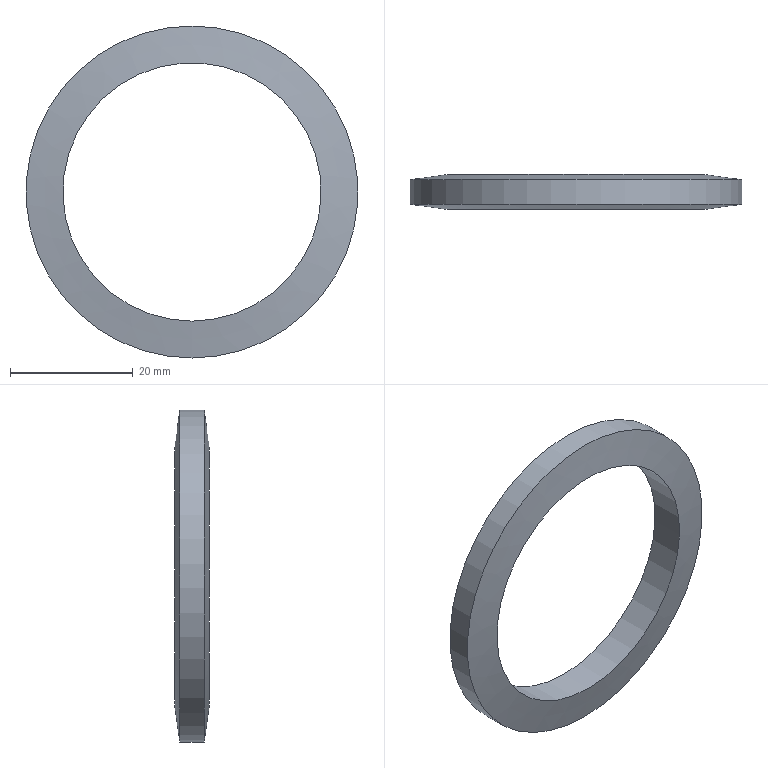Part | NX | features DATUM_CSYS 2, SKETCH 1, SWP104 1 | 1 solid | 4 faces | box 54 x 5.63 x 54 mm | volume 4326 mm3 | cone 2 | cylinder 2 | commonest cylinder face diameters 42 x1 54 x1
STEP:
#1=CARTESIAN_POINT('',(0.,-2.815,-21.));
#2=VERTEX_POINT('',#1);
#3=CARTESIAN_POINT('',(0.,-2.815,0.));
#4=DIRECTION('',(0.,-1.,0.));
#5=DIRECTION('',(0.,0.,-1.));
#6=AXIS2_PLACEMENT_3D('',#3,#4,#5);
#7=CIRCLE('',#6,21.);
#8=EDGE_CURVE('',#2,#2,#7,.T.);
#9=ORIENTED_EDGE('',*,*,#8,.F.);
#10=EDGE_LOOP('',(#9));
#11=FACE_BOUND('',#10,.T.);
#12=CARTESIAN_POINT('',(0.,-2.,-27.));
#13=VERTEX_POINT('',#12);
#14=CARTESIAN_POINT('',(0.,-2.,0.));
#15=DIRECTION('',(0.,-1.,0.));
#16=DIRECTION('',(0.,0.,-1.));
#17=AXIS2_PLACEMENT_3D('',#14,#15,#16);
#18=CIRCLE('',#17,27.);
#19=EDGE_CURVE('',#13,#13,#18,.T.);
#20=ORIENTED_EDGE('',*,*,#19,.T.);
#21=EDGE_LOOP('',(#20));
#22=FACE_BOUND('',#21,.T.);
#23=CARTESIAN_POINT('',(0.,-2.,0.));
#24=DIRECTION('',(0.,1.,0.));
#25=DIRECTION('',(0.,0.,1.));
#26=AXIS2_PLACEMENT_3D('',#23,#24,#25);
#27=CONICAL_SURFACE('',#26,27.,1.436);
#28=ADVANCED_FACE('',(#11,#22),#27,.T.);
#29=CARTESIAN_POINT('',(0.,2.815,-21.));
#30=VERTEX_POINT('',#29);
#31=CARTESIAN_POINT('',(0.,2.815,0.));
#32=DIRECTION('',(0.,-1.,0.));
#33=DIRECTION('',(0.,0.,-1.));
#34=AXIS2_PLACEMENT_3D('',#31,#32,#33);
#35=CIRCLE('',#34,21.);
#36=EDGE_CURVE('',#30,#30,#35,.T.);
#37=ORIENTED_EDGE('',*,*,#36,.F.);
#38=EDGE_LOOP('',(#37));
#39=FACE_BOUND('',#38,.T.);
#40=ORIENTED_EDGE('',*,*,#8,.T.);
#41=EDGE_LOOP('',(#40));
#42=FACE_BOUND('',#41,.T.);
#43=CARTESIAN_POINT('',(0.,0.,0.));
#44=DIRECTION('',(0.,-1.,0.));
#45=DIRECTION('',(0.,0.,-1.));
#46=AXIS2_PLACEMENT_3D('',#43,#44,#45);
#47=CYLINDRICAL_SURFACE('',#46,21.);
#48=ADVANCED_FACE('',(#39,#42),#47,.F.);
#49=CARTESIAN_POINT('',(0.,2.,-27.));
#50=VERTEX_POINT('',#49);
#51=CARTESIAN_POINT('',(0.,2.,0.));
#52=DIRECTION('',(0.,-1.,0.));
#53=DIRECTION('',(0.,0.,-1.));
#54=AXIS2_PLACEMENT_3D('',#51,#52,#53);
#55=CIRCLE('',#54,27.);
#56=EDGE_CURVE('',#50,#50,#55,.T.);
#57=ORIENTED_EDGE('',*,*,#56,.F.);
#58=EDGE_LOOP('',(#57));
#59=FACE_BOUND('',#58,.T.);
#60=ORIENTED_EDGE('',*,*,#36,.T.);
#61=EDGE_LOOP('',(#60));
#62=FACE_BOUND('',#61,.T.);
#63=CARTESIAN_POINT('',(0.,2.815,0.));
#64=DIRECTION('',(0.,-1.,0.));
#65=DIRECTION('',(0.,0.,-1.));
#66=AXIS2_PLACEMENT_3D('',#63,#64,#65);
#67=CONICAL_SURFACE('',#66,21.,1.436);
#68=ADVANCED_FACE('',(#59,#62),#67,.T.);
#69=ORIENTED_EDGE('',*,*,#19,.F.);
#70=EDGE_LOOP('',(#69));
#71=FACE_BOUND('',#70,.T.);
#72=ORIENTED_EDGE('',*,*,#56,.T.);
#73=EDGE_LOOP('',(#72));
#74=FACE_BOUND('',#73,.T.);
#75=CARTESIAN_POINT('',(0.,0.,0.));
#76=DIRECTION('',(0.,-1.,0.));
#77=DIRECTION('',(0.,0.,-1.));
#78=AXIS2_PLACEMENT_3D('',#75,#76,#77);
#79=CYLINDRICAL_SURFACE('',#78,27.);
#80=ADVANCED_FACE('',(#71,#74),#79,.T.);
#81=CLOSED_SHELL('',(#28,#48,#68,#80));
#82=MANIFOLD_SOLID_BREP('',#81);
#83=(LENGTH_UNIT()NAMED_UNIT(*)SI_UNIT(.MILLI.,.METRE.));
#84=UNCERTAINTY_MEASURE_WITH_UNIT(LENGTH_MEASURE(0.00001),#83,'','');
#85=(NAMED_UNIT(*)PLANE_ANGLE_UNIT()SI_UNIT($,.RADIAN.));
#86=(NAMED_UNIT(*)SI_UNIT($,.STERADIAN.)SOLID_ANGLE_UNIT());
#87=(GEOMETRIC_REPRESENTATION_CONTEXT(3)GLOBAL_UNCERTAINTY_ASSIGNED_CONTEXT((#84))GLOBAL_UNIT_ASSIGNED_CONTEXT((#83,#85,#86))REPRESENTATION_CONTEXT('',''));
#88=ADVANCED_BREP_SHAPE_REPRESENTATION('',(#82),#87);